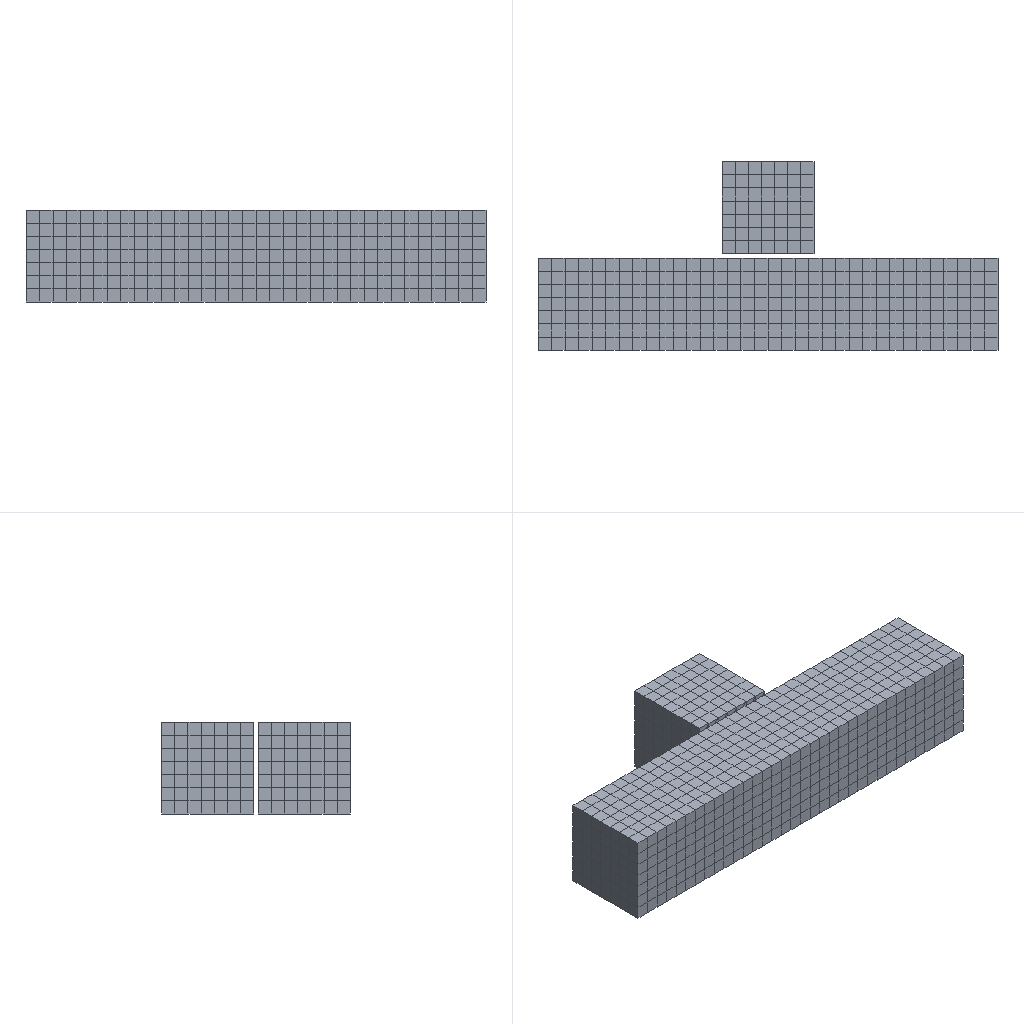Simulation study | ansys workbench
Ansys APDL input file, long lists of numbers shortened:
/batch
/config,noeldb,1     ! force off writing results to database
*get,_wallstrt,active,,time,wall
! ANSYS input file written by Workbench version 2023 R1
! File used for geometry attach:
/title,E1.7.2--Static Structural (B5)
! ****** Begin Custom Load Command Snippet ******
/COM, ACT Extensions:
/COM,     LSDYNA, 2023.1
/COM,/COM,     ANSYSMotion, 2023.1
/COM,
! ****** End   Custom Load Command Snippet ******
*DIM,_wb_ProjectScratch_dir,string,248
_wb_ProjectScratch_dir(1) = ''
*DIM,_wb_SolverFiles_dir,string,248
_wb_SolverFiles_dir(1) = ''
*DIM,_wb_userfiles_dir,string,248
_wb_userfiles_dir(1) = ''
/com,--- Data in consistent NMM units. See Solving Units in the help system for more information.
/units,MPA
/nopr
/wb,file,start              !  signify a WB generated input file
/prep7
! Turn off shape checking because checks already performed inside WB mesher.
! See help system for more information.
SHPP,OFF,,NOWARN
/nolist
etcon,set             ! allow ANSYS to choose best KEYOP's for 180x elements, resets any applicable keyopt to MAPDL defaults
/com,*********** Nodes for the whole assembly ***********
nblock,3,,11211
(1i9,3e20.9e3)
        1     2.857142857E+04     1.928571429E+03     1.428571429E+03
! (10191 more lines like these left out)
-1
/wb,elem,start            !  set before creation of elements
/com,*********** Elements for Body 1 "1" ***********
et,1,186
keyo,1,2,1          ! set full integration on SOLID186
eblock,19,solid,,1666
(19i9)
        1        1        1        1        0        0        0        0       20        0      344     1857     3898     3566     3528     3242     4096     3565     3559
! (3331 more lines like these left out)
-1
/com,*********** Elements for Body 2 "2" ***********
et,2,186
keyo,2,2,1          ! set full integration on SOLID186
eblock,19,solid,,343
(19i9)
        2        2        2        2        0        0        0        0       20        0        1        1      452      465      471      252      463      464      507
! (685 more lines like these left out)
-1
/wb,elem,end               !  done creating elements
/com,*********** Send User Defined Coordinate System(s) ***********
csys,0
toffst,273.15,  ! Temperature offset from absolute zero
/com,*********** Set Reference Temperature ***********
tref,22.
/wb,mat,start              !  starting to send materials
/com,*********** Send Materials ***********
Temperature = 'TEMP' ! Temperature
MP,DENS,1,7.85e-09,	! tonne mm^-3
MP,ALPX,1,1.2e-05,	! C^-1
MP,C,1,434000000,	! mm^2 s^-2 C^-1
MP,KXX,1,60.5,	! tonne mm s^-3 C^-1
MP,RSVX,1,0.00017,	! ohm mm
MP,EX,1,200000,	! tonne s^-2 mm^-1
MP,NUXY,1,0.3,
MP,MURX,1,10000,
Temperature = 'TEMP' ! Temperature
MP,DENS,2,7.85e-09,	! tonne mm^-3
MP,ALPX,2,1.2e-05,	! C^-1
MP,C,2,434000000,	! mm^2 s^-2 C^-1
MP,KXX,2,60.5,	! tonne mm s^-3 C^-1
MP,RSVX,2,0.00017,	! ohm mm
MP,EX,2,200000,	! tonne s^-2 mm^-1
MP,NUXY,2,0.3,
MP,MURX,2,10000,
/wb,mat,end                !  done sending materials
!************************* Model Summary ********************
!1,	Structural Steel,	matid,	1
!2,	Structural Steel,	matid,	2
!************************* End Model Summary ********************
! get the diagonal of the bounding box. Needed later for other things
*get,_xmin,node,,mnloc,x
*get,_ymin,node,,mnloc,y
*get,_zmin,node,,mnloc,z
*get,_xmax,node,,mxloc,x
*get,_ymax,node,,mxloc,y
*get,_zmax,node,,mxloc,z
_ASMDIAG=(_xmax-_xmin)*(_xmax-_xmin)+(_ymax-_ymin)*(_ymax-_ymin)+(_zmax-_zmin)*(_zmax-_zmin)
_ASMDIAG=SQRT(_ASMDIAG)
/wb,contact,start          !  starting to send contact
/com,*********** Create Contact "No Separation - 2 To 1" ***********
/com,            Real Constant Set For Above Contact Is 4 & 3
*set,tid,4
*set,cid,3
r,tid
r,cid
et,tid,170
et,cid,174
eblock,10,,,49
(15i9)
     3354        4        4        4        0      465      471      507      464     1776     1788     1774     1773
! (48 more lines like these left out)
-1
eblock,10,,,49
(15i9)
     3403        3        3        3        0      465      471      507      464     1776     1788     1774     1773
! (48 more lines like these left out)
-1
eblock,10,,,238
(15i9)
     3452        3        4        3        0     3514     3579     3578     3515     9111     9237     9113     9110
! (237 more lines like these left out)
-1
eblock,10,,,238
(15i9)
     3690        4        3        4        0     3514     3579     3578     3515     9111     9237     9113     9110
! (237 more lines like these left out)
-1
keyo,cid,8,2               ! auto create asymmetric contact (from Program Controlled setting)
keyo,cid,10,0              ! adjust contact stiffness each NR iteration
keyo,cid,12,4              ! no separation always
keyo,cid,18,0              ! finite small sliding
keyo,cid,2,0               ! augmented Lagrange (from Program Controlled setting)
keyo,cid,4,0               ! on Gauss point (from Program Controlled setting)
keyo,cid,9,1               ! ignore initial gaps/penetration
keyo,cid,7,1               ! Automatic Bisection
rmod,tid,3,1.       ! FKN
rmod,tid,5,0.       ! ICONT
rmod,tid,6,0.       ! PINB
rmod,tid,10,0.      ! CNOF
rmod,tid,12,0.      ! FKT
rmod,tid,36,33      ! WB DSID
rmod,cid,3,1.       ! FKN
rmod,cid,5,0.       ! ICONT
rmod,cid,6,0.       ! PINB
rmod,cid,10,0.      ! CNOF
rmod,cid,12,0.      ! FKT
rmod,cid,36,33      ! WB DSID
nsel,all
esel,all
/wb,contact,end            !  done creating contacts
/golist
/wb,load,start             !  starting to send loads
/com,*********** Fixed Supports ***********
CMBLOCK,_FIXEDSU,NODE,      352
(8i10)
      3474      3475      3476      3477      3478      3479      3480      3481
! (43 more lines like these left out)
cmsel,s,_FIXEDSU
d,all,all
nsel,all
/com,******* Constant Zero Displacement X *******
CMBLOCK,_DISPZEROUX,NODE,      176
(8i10)
       302       303       304       305       306       307       308       309
! (21 more lines like these left out)
cmsel,s,_DISPZEROUX
d,all,ux,0
nsel,all
/com,******* Constant Zero Displacement Z *******
CMBLOCK,_DISPZEROUZ,NODE,      176
(8i10)
       302       303       304       305       306       307       308       309
! (21 more lines like these left out)
cmsel,s,_DISPZEROUZ
d,all,uz,0
nsel,all
/com,*********** Create Displacement Tables and Functions ******
*DIM,_loadvari59yp,TABLE,2,1,1,TIME
! Time values
*TAXIS,_loadvari59yp(1),1,0.,1.
! Load values
_loadvari59yp(1,1,1) = 0.
_loadvari59yp(2,1,1) = -600.
*DIM,_loadvari59yn,TABLE,2,1,1,TIME
! Time values
*TAXIS,_loadvari59yn(1),1,0.,1.
! Load values
_loadvari59yn(1,1,1) = 0.
_loadvari59yn(2,1,1) = 600.
/gst,on,on
fini
*get,_numnode,node,0,count
*get,_numelem,elem,0,count
*get, _MAXELEMNUM, elem, 0, NUM, MAX
*get, _MAXNODENUM, node, 0, NUM, MAX
*get, _MAXELEMTYPE, etyp, 0, NUM, MAX
*get, _MAXREALCONST, rcon, 0, NUM, MAX
/go
/wb,load,end               !  done creating loads
/com,--- Number of total nodes = %_numnode%
/com,--- Number of contact elements = 574
/com,--- Number of spring elements = 0
/com,--- Number of bearing elements = 0
/com,--- Number of solid elements = 2009
/com,--- Number of condensed parts = 0
/com,--- Number of total elements = %_numelem%
*get,_wallbsol,active,,time,wall
/com,****************************************************************************
/com,*************************    SOLUTION       ********************************
/com,****************************************************************************
/solu
antype,0                   ! static analysis
neqit,1,force              ! Force 1 eq iteration since only nonlinearity is bonded/no sep contact
pred,off
_thickRatio=  1     ! Ratio of thick parts in the model
eqsl,pcg,1e-8,,,,,,1
cntr,print,1               ! print out contact info and also make no initial contact an error
nldiag,cont,iter           ! print out contact info each equilibrium iteration
rescontrol,,none                 ! Do not keep any restart files
/com,****************************************************
/com,******************* SOLVE FOR LS 1 OF 1 ****************
/com,*** Set Displacements ***
CMBLOCK,_CM59UY_YP,NODE,      176
(8i10)
       302       303       304       305       306       307       308       309
! (21 more lines like these left out)
cmsel,s,_CM59UY_YP
d,all,uy,%_loadvari59yp%
nsel,all
/com,*** Component For All Non-Zero UY Displacements ***
cmsel,s,_CM59uy_yp
cm,_DISPNONZEROUY,NODE
nsel,all
/nopr
/gopr
autots,off                 ! User turned off automatic time stepping
nsub,20,20,20
time,1.
outres,erase
outres,all,none
outres,nsol,all,
outres,rsol,all
outres,eangl,all
outres,etmp,all
outres,veng,all
outres,strs,all,
outres,epel,all,
outres,eppl,all,
outres,cont,all,
! *********** WB SOLVE COMMAND ***********
! check interactive state
*get,ANSINTER_,active,,int
*if,ANSINTER_,ne,0,then
/eof
*endif
solve
/com *************** Write FE CONNECTORS *********
CEWRITE,file,ce,,INTE
/com,****************************************************
/com,*************** FINISHED SOLVE FOR LS 1 *************
*get,_wallasol,active,,time,wall
/nopr
*get,_numnode,node,0,count
*get,_numelem,elem,0,count
*get, _MAXELEMNUM, elem, 0, NUM, MAX
*get, _MAXNODENUM, node, 0, NUM, MAX,,,INTERNAL
*get, _MAXELEMTYPE, etyp, 0, NUM, MAX
*get, _MAXREALCONST, rcon, 0, NUM, MAX
*get,_NSOLTHREADS,active,0,ntfs
*get,_NSOLPROCESSES,active,0,npfs
/gopr
*get,_PCGITER,active,,solu,cgiter
/post1
xmlo,ENCODING,ISO-8859-1
xmlo,parm
/xml,parm,xml
fini
/gopr
*get,_walldone,active,,time,wall
_preptime=(_wallbsol-_wallstrt)*3600
_solvtime=(_wallasol-_wallbsol)*3600
_posttime=(_walldone-_wallasol)*3600
_totaltim=(_walldone-_wallstrt)*3600
*get,_dlbratio,active,0,solu,dlbr
*get,_combtime,active,0,solu,comb
*get,_ssmode,active,0,solu,ssmm
*get,_ndofs,active,0,solu,ndof
/com,--- Total number of nodes = %_numnode%
/com,--- Total number of elements = %_numelem%
/com,--- Element load balance ratio = %_dlbratio%
/com,--- Time to combine distributed files = %_combtime%
/com,--- Sparse memory mode = %_ssmode%
/com,--- Number of DOF = %_ndofs%
/wb,file,end               ! done with WB generated input